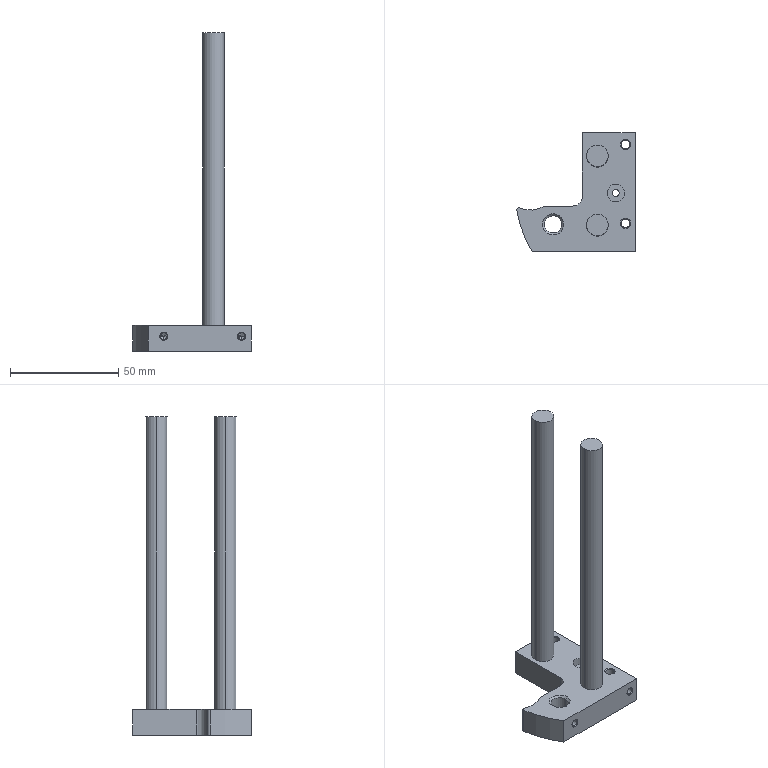Part | STEP file | 1 solid | 62 faces | box 54.828 x 55 x 147.5 mm | volume 42895 mm3 | cone 27 | cylinder 24 | plane 11 | commonest cylinder face diameters 3.2 x6 4 x4 8 x4 10 x4 6 x2 2 x1